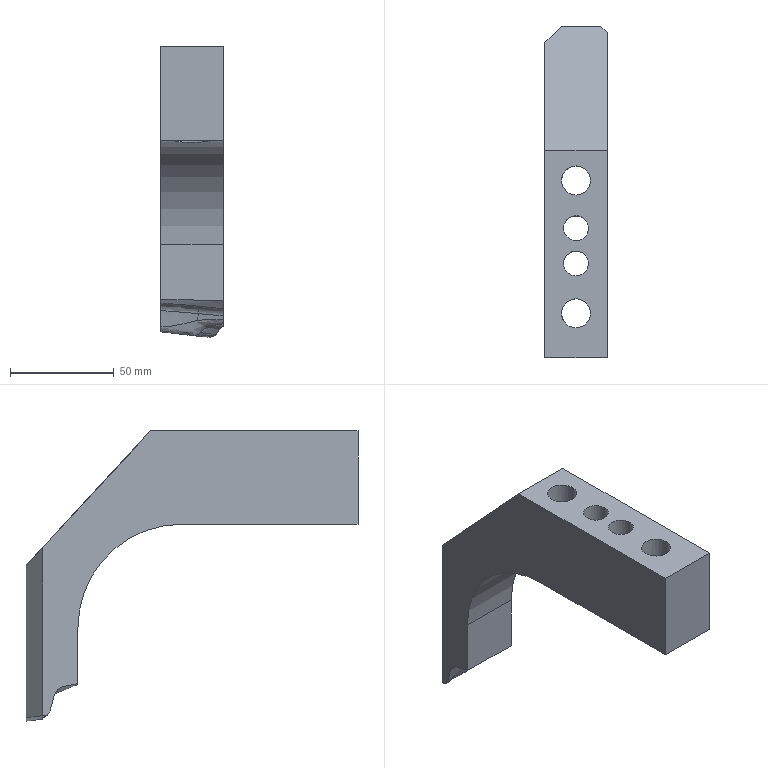Part | NX | features solid 2 | 1 solid | 30 faces | box 30.001 x 160 x 139.858 mm | volume 204254 mm3 | plane 12 | spline 11 | cylinder 7 | commonest cylinder face diameters 12 x2 14 x2 20 x2 100 x1